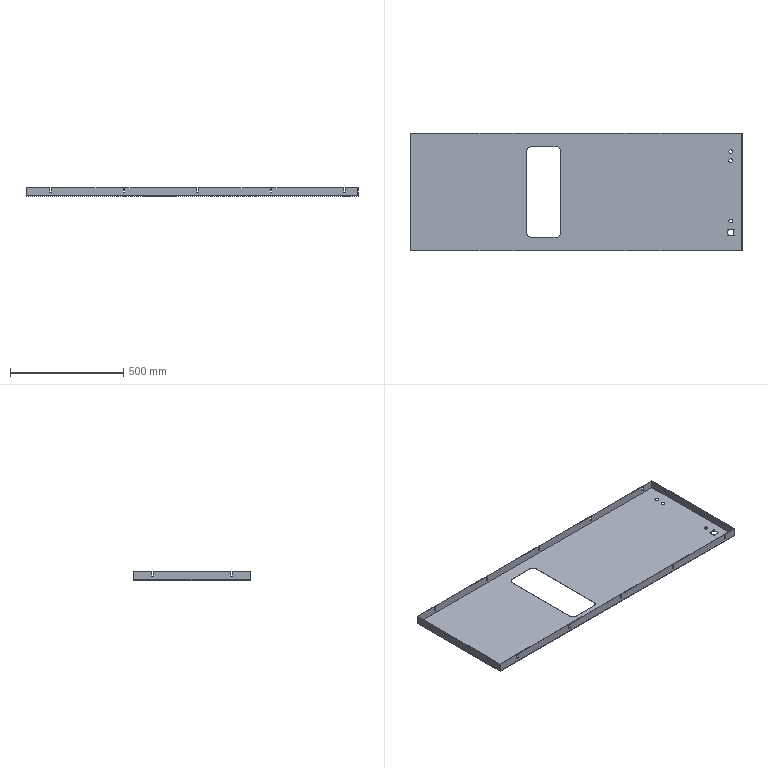Part | STEP file | ICT side seal plate | 1 solid | 94 faces | box 1468 x 518 x 38 mm | volume 1263222 mm3 | plane 56 | cylinder 38 | commonest cylinder face diameters 7 x18 2 x8 16.2 x6 40 x4 28 x2